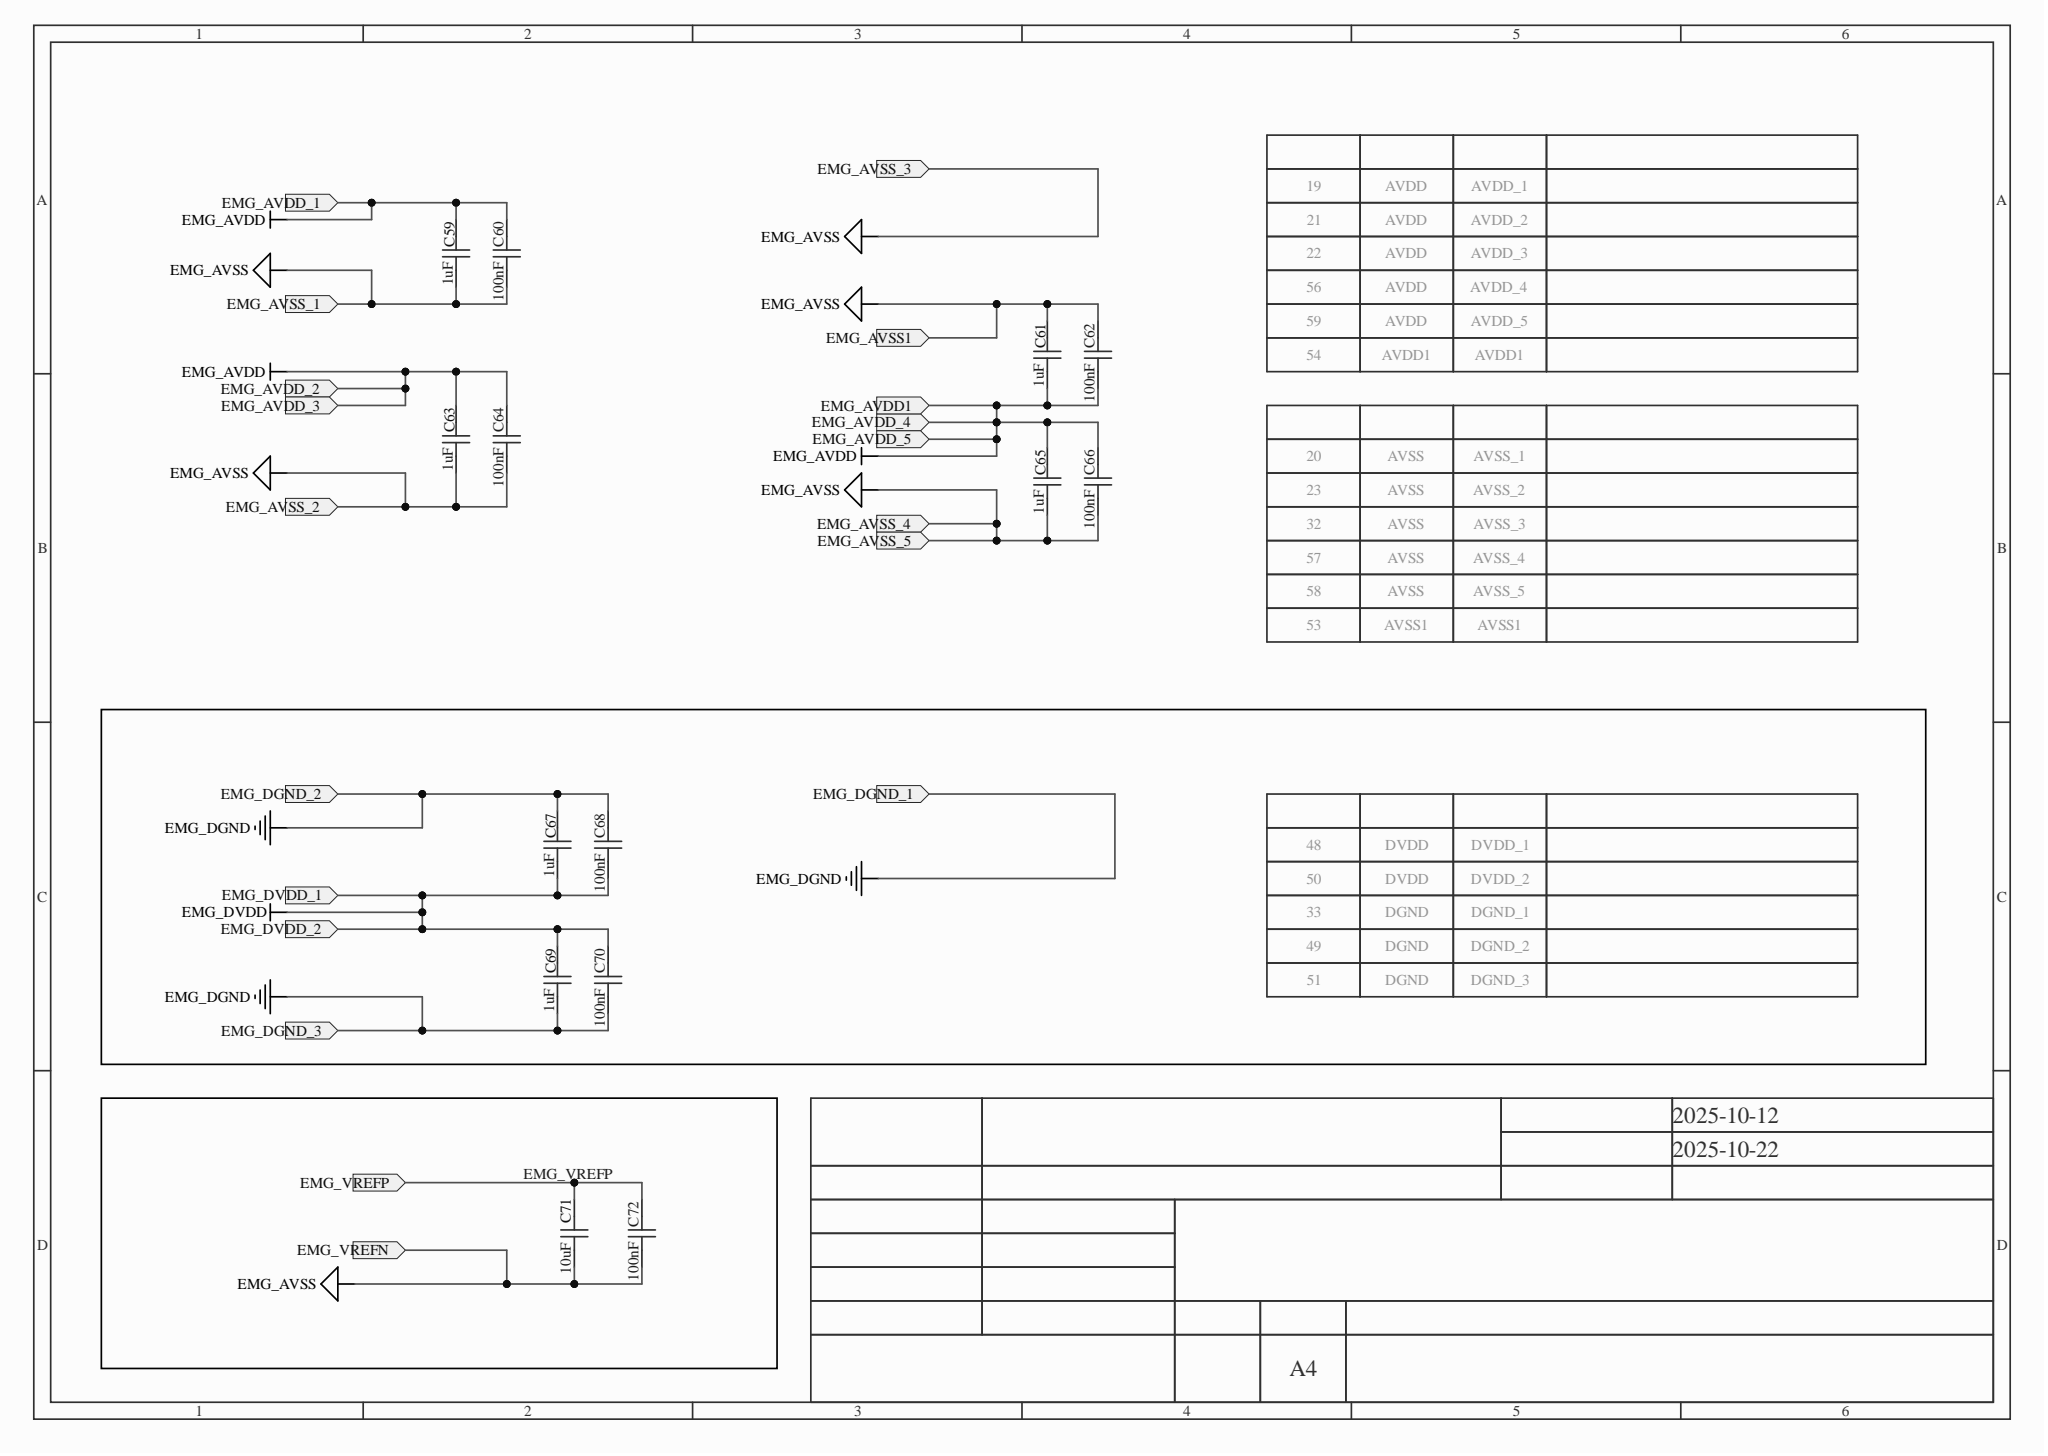Circuit board | Altium Designer | 212 parts | 123 nets | one sheet of the schematic
Parts on this sheet (reference | value | footprint):
C59 | 1uF | C0402
C60 | 100nF | C0402
C61 | 1uF | C0402
C62 | 100nF | C0402
C63 | 1uF | C0402
C64 | 100nF | C0402
C65 | 1uF | C0402
C66 | 100nF | C0402
C67 | 1uF | C0402
C68 | 100nF | C0402
C69 | 1uF | C0402
C70 | 100nF | C0402
C71 | 10uF | C0603
C72 | 100nF | C0402
Nets of these parts (net: part-pin ...):
EMG_VREFP: C71-2 C72-2
EMG_DVDD: C67-1 C68-1 C69-2 C70-2
EMG_DGND: C67-2 C68-2 C69-1 C70-1
EMG_AVSS1: C59-1 C60-1 C61-2 C62-2 C63-1 C64-1 C65-1 C66-1 C71-1 C72-1
EMG_AVDD1: C59-2 C60-2 C61-1 C62-1 C63-2 C64-2 C65-2 C66-2